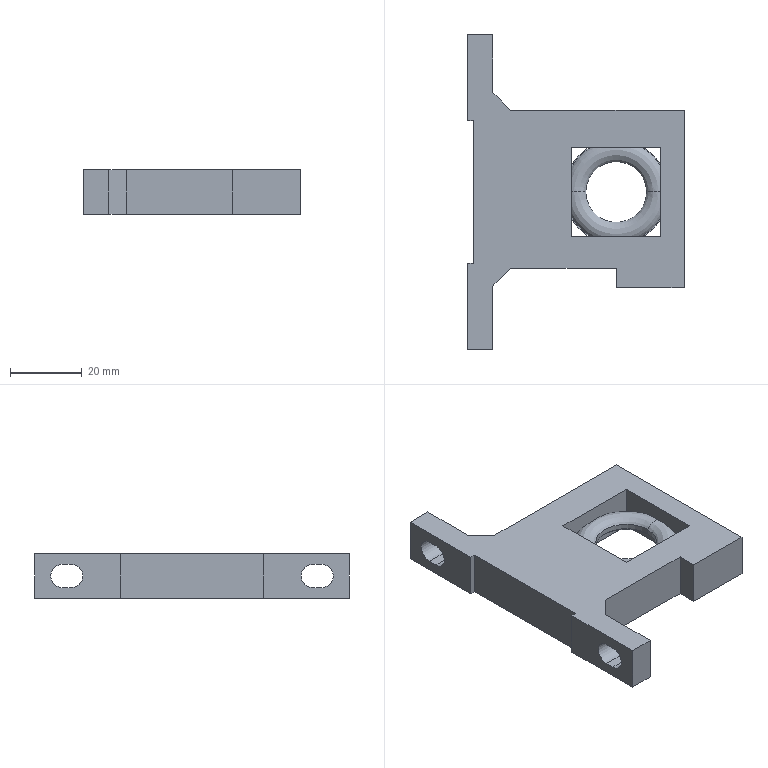Part | STEP file | T-bracket GA300T-P1 | 1 solid | 64 faces | box 60.5 x 88 x 12.5 mm | volume 30830 mm3 | plane 38 | cylinder 18 | torus 8 | commonest cylinder face diameters 6.5 x4 7 x4 7.5 x4 29.2 x4 17 x2